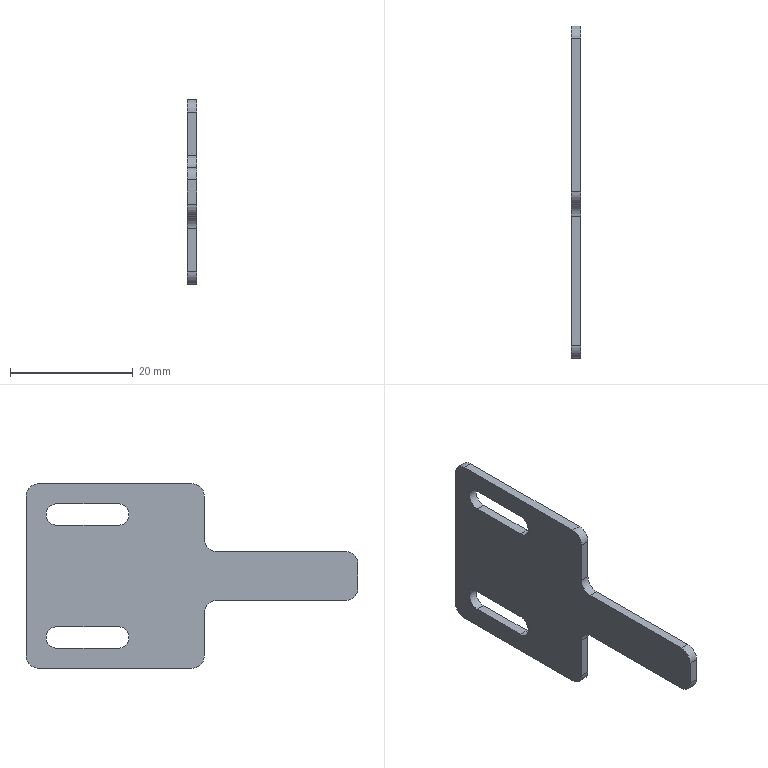Part | SolidWorks | features BaseBody 1 | 1 solid | 26 faces | box 1.5 x 54 x 30 mm | volume 1466 mm3 | plane 14 | cylinder 12 | commonest cylinder face diameters 4 x8 3.5 x4
STEP:
#1=CARTESIAN_POINT('',(-15.435,38.729,3.25));
#2=VERTEX_POINT('',#1);
#3=CARTESIAN_POINT('',(-15.435,28.729,3.25));
#4=VERTEX_POINT('',#3);
#5=CARTESIAN_POINT('',(-15.435,43.729,3.25));
#6=DIRECTION('',(0.,-1.,0.));
#7=VECTOR('',#6,1000.);
#8=LINE('',#5,#7);
#9=EDGE_CURVE('',#2,#4,#8,.T.);
#10=ORIENTED_EDGE('',*,*,#9,.F.);
#11=CARTESIAN_POINT('',(-15.435,38.729,6.75));
#12=VERTEX_POINT('',#11);
#13=CARTESIAN_POINT('',(-15.435,38.729,5.));
#14=DIRECTION('',(-1.,0.,0.));
#15=DIRECTION('',(0.,0.,-1.));
#16=AXIS2_PLACEMENT_3D('',#13,#14,#15);
#17=CIRCLE('',#16,1.75);
#18=EDGE_CURVE('',#12,#2,#17,.T.);
#19=ORIENTED_EDGE('',*,*,#18,.F.);
#20=CARTESIAN_POINT('',(-15.435,28.729,6.75));
#21=VERTEX_POINT('',#20);
#22=CARTESIAN_POINT('',(-15.435,43.729,6.75));
#23=DIRECTION('',(0.,1.,0.));
#24=VECTOR('',#23,1000.);
#25=LINE('',#22,#24);
#26=EDGE_CURVE('',#21,#12,#25,.T.);
#27=ORIENTED_EDGE('',*,*,#26,.F.);
#28=CARTESIAN_POINT('',(-15.435,28.729,5.));
#29=DIRECTION('',(-1.,0.,0.));
#30=DIRECTION('',(0.,0.,-1.));
#31=AXIS2_PLACEMENT_3D('',#28,#29,#30);
#32=CIRCLE('',#31,1.75);
#33=EDGE_CURVE('',#4,#21,#32,.T.);
#34=ORIENTED_EDGE('',*,*,#33,.F.);
#35=EDGE_LOOP('',(#10,#19,#27,#34));
#36=FACE_BOUND('',#35,.T.);
#37=CARTESIAN_POINT('',(-15.435,38.729,23.25));
#38=VERTEX_POINT('',#37);
#39=CARTESIAN_POINT('',(-15.435,28.729,23.25));
#40=VERTEX_POINT('',#39);
#41=CARTESIAN_POINT('',(-15.435,43.729,23.25));
#42=DIRECTION('',(0.,-1.,0.));
#43=VECTOR('',#42,1000.);
#44=LINE('',#41,#43);
#45=EDGE_CURVE('',#38,#40,#44,.T.);
#46=ORIENTED_EDGE('',*,*,#45,.F.);
#47=CARTESIAN_POINT('',(-15.435,38.729,26.75));
#48=VERTEX_POINT('',#47);
#49=CARTESIAN_POINT('',(-15.435,38.729,25.));
#50=DIRECTION('',(-1.,0.,0.));
#51=DIRECTION('',(0.,0.,-1.));
#52=AXIS2_PLACEMENT_3D('',#49,#50,#51);
#53=CIRCLE('',#52,1.75);
#54=EDGE_CURVE('',#48,#38,#53,.T.);
#55=ORIENTED_EDGE('',*,*,#54,.F.);
#56=CARTESIAN_POINT('',(-15.435,28.729,26.75));
#57=VERTEX_POINT('',#56);
#58=CARTESIAN_POINT('',(-15.435,43.729,26.75));
#59=DIRECTION('',(0.,1.,0.));
#60=VECTOR('',#59,1000.);
#61=LINE('',#58,#60);
#62=EDGE_CURVE('',#57,#48,#61,.T.);
#63=ORIENTED_EDGE('',*,*,#62,.F.);
#64=CARTESIAN_POINT('',(-15.435,28.729,25.));
#65=DIRECTION('',(-1.,0.,0.));
#66=DIRECTION('',(0.,0.,-1.));
#67=AXIS2_PLACEMENT_3D('',#64,#65,#66);
#68=CIRCLE('',#67,1.75);
#69=EDGE_CURVE('',#40,#57,#68,.T.);
#70=ORIENTED_EDGE('',*,*,#69,.F.);
#71=EDGE_LOOP('',(#46,#55,#63,#70));
#72=FACE_BOUND('',#71,.T.);
#73=CARTESIAN_POINT('',(-15.435,14.729,9.));
#74=VERTEX_POINT('',#73);
#75=CARTESIAN_POINT('',(-15.435,14.729,2.));
#76=VERTEX_POINT('',#75);
#77=CARTESIAN_POINT('',(-15.435,14.729,30.));
#78=DIRECTION('',(0.,0.,-1.));
#79=VECTOR('',#78,1000.);
#80=LINE('',#77,#79);
#81=EDGE_CURVE('',#74,#76,#80,.T.);
#82=ORIENTED_EDGE('',*,*,#81,.F.);
#83=CARTESIAN_POINT('',(-15.435,12.729,11.));
#84=VERTEX_POINT('',#83);
#85=CARTESIAN_POINT('',(-15.435,12.729,9.));
#86=DIRECTION('',(-1.,0.,0.));
#87=DIRECTION('',(0.,-1.,0.));
#88=AXIS2_PLACEMENT_3D('',#85,#86,#87);
#89=CIRCLE('',#88,2.);
#90=EDGE_CURVE('',#84,#74,#89,.T.);
#91=ORIENTED_EDGE('',*,*,#90,.F.);
#92=CARTESIAN_POINT('',(-15.435,-8.271,11.));
#93=VERTEX_POINT('',#92);
#94=CARTESIAN_POINT('',(-15.435,43.729,11.));
#95=DIRECTION('',(0.,1.,0.));
#96=VECTOR('',#95,1000.);
#97=LINE('',#94,#96);
#98=EDGE_CURVE('',#93,#84,#97,.T.);
#99=ORIENTED_EDGE('',*,*,#98,.F.);
#100=CARTESIAN_POINT('',(-15.435,-10.271,13.));
#101=VERTEX_POINT('',#100);
#102=CARTESIAN_POINT('',(-15.435,-8.271,13.));
#103=DIRECTION('',(1.,0.,0.));
#104=DIRECTION('',(0.,0.,-1.));
#105=AXIS2_PLACEMENT_3D('',#102,#103,#104);
#106=CIRCLE('',#105,2.);
#107=EDGE_CURVE('',#101,#93,#106,.T.);
#108=ORIENTED_EDGE('',*,*,#107,.F.);
#109=CARTESIAN_POINT('',(-15.435,-10.271,17.));
#110=VERTEX_POINT('',#109);
#111=CARTESIAN_POINT('',(-15.435,-10.271,30.));
#112=DIRECTION('',(0.,0.,-1.));
#113=VECTOR('',#112,1000.);
#114=LINE('',#111,#113);
#115=EDGE_CURVE('',#110,#101,#114,.T.);
#116=ORIENTED_EDGE('',*,*,#115,.F.);
#117=CARTESIAN_POINT('',(-15.435,-8.271,19.));
#118=VERTEX_POINT('',#117);
#119=CARTESIAN_POINT('',(-15.435,-8.271,17.));
#120=DIRECTION('',(1.,0.,0.));
#121=DIRECTION('',(0.,0.,-1.));
#122=AXIS2_PLACEMENT_3D('',#119,#120,#121);
#123=CIRCLE('',#122,2.);
#124=EDGE_CURVE('',#118,#110,#123,.T.);
#125=ORIENTED_EDGE('',*,*,#124,.F.);
#126=CARTESIAN_POINT('',(-15.435,12.729,19.));
#127=VERTEX_POINT('',#126);
#128=CARTESIAN_POINT('',(-15.435,43.729,19.));
#129=DIRECTION('',(0.,-1.,0.));
#130=VECTOR('',#129,1000.);
#131=LINE('',#128,#130);
#132=EDGE_CURVE('',#127,#118,#131,.T.);
#133=ORIENTED_EDGE('',*,*,#132,.F.);
#134=CARTESIAN_POINT('',(-15.435,14.729,21.));
#135=VERTEX_POINT('',#134);
#136=CARTESIAN_POINT('',(-15.435,12.729,21.));
#137=DIRECTION('',(-1.,0.,0.));
#138=DIRECTION('',(0.,-1.,0.));
#139=AXIS2_PLACEMENT_3D('',#136,#137,#138);
#140=CIRCLE('',#139,2.);
#141=EDGE_CURVE('',#135,#127,#140,.T.);
#142=ORIENTED_EDGE('',*,*,#141,.F.);
#143=CARTESIAN_POINT('',(-15.435,14.729,28.));
#144=VERTEX_POINT('',#143);
#145=CARTESIAN_POINT('',(-15.435,14.729,30.));
#146=DIRECTION('',(0.,0.,-1.));
#147=VECTOR('',#146,1000.);
#148=LINE('',#145,#147);
#149=EDGE_CURVE('',#144,#135,#148,.T.);
#150=ORIENTED_EDGE('',*,*,#149,.F.);
#151=CARTESIAN_POINT('',(-15.435,16.729,30.));
#152=VERTEX_POINT('',#151);
#153=CARTESIAN_POINT('',(-15.435,16.729,28.));
#154=DIRECTION('',(1.,0.,0.));
#155=DIRECTION('',(0.,1.,0.));
#156=AXIS2_PLACEMENT_3D('',#153,#154,#155);
#157=CIRCLE('',#156,2.);
#158=EDGE_CURVE('',#152,#144,#157,.T.);
#159=ORIENTED_EDGE('',*,*,#158,.F.);
#160=CARTESIAN_POINT('',(-15.435,41.729,30.));
#161=VERTEX_POINT('',#160);
#162=CARTESIAN_POINT('',(-15.435,43.729,30.));
#163=DIRECTION('',(0.,-1.,0.));
#164=VECTOR('',#163,1000.);
#165=LINE('',#162,#164);
#166=EDGE_CURVE('',#161,#152,#165,.T.);
#167=ORIENTED_EDGE('',*,*,#166,.F.);
#168=CARTESIAN_POINT('',(-15.435,43.729,28.));
#169=VERTEX_POINT('',#168);
#170=CARTESIAN_POINT('',(-15.435,41.729,28.));
#171=DIRECTION('',(1.,0.,0.));
#172=DIRECTION('',(0.,0.,1.));
#173=AXIS2_PLACEMENT_3D('',#170,#171,#172);
#174=CIRCLE('',#173,2.);
#175=EDGE_CURVE('',#169,#161,#174,.T.);
#176=ORIENTED_EDGE('',*,*,#175,.F.);
#177=CARTESIAN_POINT('',(-15.435,43.729,2.));
#178=VERTEX_POINT('',#177);
#179=CARTESIAN_POINT('',(-15.435,43.729,30.));
#180=DIRECTION('',(0.,0.,1.));
#181=VECTOR('',#180,1000.);
#182=LINE('',#179,#181);
#183=EDGE_CURVE('',#178,#169,#182,.T.);
#184=ORIENTED_EDGE('',*,*,#183,.F.);
#185=CARTESIAN_POINT('',(-15.435,41.729,0.));
#186=VERTEX_POINT('',#185);
#187=CARTESIAN_POINT('',(-15.435,41.729,2.));
#188=DIRECTION('',(1.,0.,0.));
#189=DIRECTION('',(0.,0.,-1.));
#190=AXIS2_PLACEMENT_3D('',#187,#188,#189);
#191=CIRCLE('',#190,2.);
#192=EDGE_CURVE('',#186,#178,#191,.T.);
#193=ORIENTED_EDGE('',*,*,#192,.F.);
#194=CARTESIAN_POINT('',(-15.435,16.729,0.));
#195=VERTEX_POINT('',#194);
#196=CARTESIAN_POINT('',(-15.435,43.729,0.));
#197=DIRECTION('',(0.,1.,0.));
#198=VECTOR('',#197,1000.);
#199=LINE('',#196,#198);
#200=EDGE_CURVE('',#195,#186,#199,.T.);
#201=ORIENTED_EDGE('',*,*,#200,.F.);
#202=CARTESIAN_POINT('',(-15.435,16.729,2.));
#203=DIRECTION('',(1.,0.,0.));
#204=DIRECTION('',(0.,-1.,0.));
#205=AXIS2_PLACEMENT_3D('',#202,#203,#204);
#206=CIRCLE('',#205,2.);
#207=EDGE_CURVE('',#76,#195,#206,.T.);
#208=ORIENTED_EDGE('',*,*,#207,.F.);
#209=EDGE_LOOP('',(#82,#91,#99,#108,#116,#125,#133,#142,#150,#159,#167,#176,#184,#193,#201,#208));
#210=FACE_OUTER_BOUND('',#209,.T.);
#211=CARTESIAN_POINT('',(-15.435,43.729,30.));
#212=DIRECTION('',(1.,0.,0.));
#213=DIRECTION('',(0.,1.,0.));
#214=AXIS2_PLACEMENT_3D('',#211,#212,#213);
#215=PLANE('',#214);
#216=ADVANCED_FACE('',(#36,#72,#210),#215,.F.);
#217=CARTESIAN_POINT('',(-13.935,28.729,6.75));
#218=VERTEX_POINT('',#217);
#219=CARTESIAN_POINT('',(-43.935,28.729,6.75));
#220=DIRECTION('',(-1.,0.,0.));
#221=VECTOR('',#220,1000.);
#222=LINE('',#219,#221);
#223=EDGE_CURVE('',#218,#21,#222,.T.);
#224=ORIENTED_EDGE('',*,*,#223,.F.);
#225=CARTESIAN_POINT('',(-13.935,28.729,3.25));
#226=VERTEX_POINT('',#225);
#227=CARTESIAN_POINT('',(-13.935,28.729,5.));
#228=DIRECTION('',(-1.,0.,0.));
#229=DIRECTION('',(0.,0.,-1.));
#230=AXIS2_PLACEMENT_3D('',#227,#228,#229);
#231=CIRCLE('',#230,1.75);
#232=EDGE_CURVE('',#226,#218,#231,.T.);
#233=ORIENTED_EDGE('',*,*,#232,.F.);
#234=CARTESIAN_POINT('',(-43.935,28.729,3.25));
#235=DIRECTION('',(1.,0.,0.));
#236=VECTOR('',#235,1000.);
#237=LINE('',#234,#236);
#238=EDGE_CURVE('',#4,#226,#237,.T.);
#239=ORIENTED_EDGE('',*,*,#238,.F.);
#240=ORIENTED_EDGE('',*,*,#33,.T.);
#241=EDGE_LOOP('',(#224,#233,#239,#240));
#242=FACE_OUTER_BOUND('',#241,.T.);
#243=CARTESIAN_POINT('',(-43.935,28.729,5.));
#244=DIRECTION('',(1.,0.,0.));
#245=DIRECTION('',(0.,0.,-1.));
#246=AXIS2_PLACEMENT_3D('',#243,#244,#245);
#247=CYLINDRICAL_SURFACE('',#246,1.75);
#248=ADVANCED_FACE('',(#242),#247,.F.);
#249=ORIENTED_EDGE('',*,*,#238,.T.);
#250=CARTESIAN_POINT('',(-13.935,38.729,3.25));
#251=VERTEX_POINT('',#250);
#252=CARTESIAN_POINT('',(-13.935,38.729,3.25));
#253=DIRECTION('',(0.,-1.,0.));
#254=VECTOR('',#253,1000.);
#255=LINE('',#252,#254);
#256=EDGE_CURVE('',#251,#226,#255,.T.);
#257=ORIENTED_EDGE('',*,*,#256,.F.);
#258=CARTESIAN_POINT('',(-43.935,38.729,3.25));
#259=DIRECTION('',(1.,0.,0.));
#260=VECTOR('',#259,1000.);
#261=LINE('',#258,#260);
#262=EDGE_CURVE('',#2,#251,#261,.T.);
#263=ORIENTED_EDGE('',*,*,#262,.F.);
#264=ORIENTED_EDGE('',*,*,#9,.T.);
#265=EDGE_LOOP('',(#249,#257,#263,#264));
#266=FACE_OUTER_BOUND('',#265,.T.);
#267=CARTESIAN_POINT('',(-43.935,38.729,3.25));
#268=DIRECTION('',(0.,0.,-1.));
#269=DIRECTION('',(0.,1.,0.));
#270=AXIS2_PLACEMENT_3D('',#267,#268,#269);
#271=PLANE('',#270);
#272=ADVANCED_FACE('',(#266),#271,.F.);
#273=ORIENTED_EDGE('',*,*,#262,.T.);
#274=CARTESIAN_POINT('',(-13.935,38.729,6.75));
#275=VERTEX_POINT('',#274);
#276=CARTESIAN_POINT('',(-13.935,38.729,5.));
#277=DIRECTION('',(-1.,0.,0.));
#278=DIRECTION('',(0.,0.,-1.));
#279=AXIS2_PLACEMENT_3D('',#276,#277,#278);
#280=CIRCLE('',#279,1.75);
#281=EDGE_CURVE('',#275,#251,#280,.T.);
#282=ORIENTED_EDGE('',*,*,#281,.F.);
#283=CARTESIAN_POINT('',(-43.935,38.729,6.75));
#284=DIRECTION('',(1.,0.,0.));
#285=VECTOR('',#284,1000.);
#286=LINE('',#283,#285);
#287=EDGE_CURVE('',#12,#275,#286,.T.);
#288=ORIENTED_EDGE('',*,*,#287,.F.);
#289=ORIENTED_EDGE('',*,*,#18,.T.);
#290=EDGE_LOOP('',(#273,#282,#288,#289));
#291=FACE_OUTER_BOUND('',#290,.T.);
#292=CARTESIAN_POINT('',(-43.935,38.729,5.));
#293=DIRECTION('',(1.,0.,0.));
#294=DIRECTION('',(0.,0.,-1.));
#295=AXIS2_PLACEMENT_3D('',#292,#293,#294);
#296=CYLINDRICAL_SURFACE('',#295,1.75);
#297=ADVANCED_FACE('',(#291),#296,.F.);
#298=ORIENTED_EDGE('',*,*,#287,.T.);
#299=CARTESIAN_POINT('',(-13.935,38.729,6.75));
#300=DIRECTION('',(0.,1.,0.));
#301=VECTOR('',#300,1000.);
#302=LINE('',#299,#301);
#303=EDGE_CURVE('',#218,#275,#302,.T.);
#304=ORIENTED_EDGE('',*,*,#303,.F.);
#305=ORIENTED_EDGE('',*,*,#223,.T.);
#306=ORIENTED_EDGE('',*,*,#26,.T.);
#307=EDGE_LOOP('',(#298,#304,#305,#306));
#308=FACE_OUTER_BOUND('',#307,.T.);
#309=CARTESIAN_POINT('',(-43.935,38.729,6.75));
#310=DIRECTION('',(0.,0.,1.));
#311=DIRECTION('',(0.,-1.,0.));
#312=AXIS2_PLACEMENT_3D('',#309,#310,#311);
#313=PLANE('',#312);
#314=ADVANCED_FACE('',(#308),#313,.F.);
#315=CARTESIAN_POINT('',(-13.935,28.729,26.75));
#316=VERTEX_POINT('',#315);
#317=CARTESIAN_POINT('',(-43.935,28.729,26.75));
#318=DIRECTION('',(-1.,0.,0.));
#319=VECTOR('',#318,1000.);
#320=LINE('',#317,#319);
#321=EDGE_CURVE('',#316,#57,#320,.T.);
#322=ORIENTED_EDGE('',*,*,#321,.F.);
#323=CARTESIAN_POINT('',(-13.935,28.729,23.25));
#324=VERTEX_POINT('',#323);
#325=CARTESIAN_POINT('',(-13.935,28.729,25.));
#326=DIRECTION('',(-1.,0.,0.));
#327=DIRECTION('',(0.,0.,-1.));
#328=AXIS2_PLACEMENT_3D('',#325,#326,#327);
#329=CIRCLE('',#328,1.75);
#330=EDGE_CURVE('',#324,#316,#329,.T.);
#331=ORIENTED_EDGE('',*,*,#330,.F.);
#332=CARTESIAN_POINT('',(-43.935,28.729,23.25));
#333=DIRECTION('',(1.,0.,0.));
#334=VECTOR('',#333,1000.);
#335=LINE('',#332,#334);
#336=EDGE_CURVE('',#40,#324,#335,.T.);
#337=ORIENTED_EDGE('',*,*,#336,.F.);
#338=ORIENTED_EDGE('',*,*,#69,.T.);
#339=EDGE_LOOP('',(#322,#331,#337,#338));
#340=FACE_OUTER_BOUND('',#339,.T.);
#341=CARTESIAN_POINT('',(-43.935,28.729,25.));
#342=DIRECTION('',(1.,0.,0.));
#343=DIRECTION('',(0.,0.,-1.));
#344=AXIS2_PLACEMENT_3D('',#341,#342,#343);
#345=CYLINDRICAL_SURFACE('',#344,1.75);
#346=ADVANCED_FACE('',(#340),#345,.F.);
#347=ORIENTED_EDGE('',*,*,#336,.T.);
#348=CARTESIAN_POINT('',(-13.935,38.729,23.25));
#349=VERTEX_POINT('',#348);
#350=CARTESIAN_POINT('',(-13.935,38.729,23.25));
#351=DIRECTION('',(0.,-1.,0.));
#352=VECTOR('',#351,1000.);
#353=LINE('',#350,#352);
#354=EDGE_CURVE('',#349,#324,#353,.T.);
#355=ORIENTED_EDGE('',*,*,#354,.F.);
#356=CARTESIAN_POINT('',(-43.935,38.729,23.25));
#357=DIRECTION('',(1.,0.,0.));
#358=VECTOR('',#357,1000.);
#359=LINE('',#356,#358);
#360=EDGE_CURVE('',#38,#349,#359,.T.);
#361=ORIENTED_EDGE('',*,*,#360,.F.);
#362=ORIENTED_EDGE('',*,*,#45,.T.);
#363=EDGE_LOOP('',(#347,#355,#361,#362));
#364=FACE_OUTER_BOUND('',#363,.T.);
#365=CARTESIAN_POINT('',(-43.935,38.729,23.25));
#366=DIRECTION('',(0.,0.,-1.));
#367=DIRECTION('',(0.,1.,0.));
#368=AXIS2_PLACEMENT_3D('',#365,#366,#367);
#369=PLANE('',#368);
#370=ADVANCED_FACE('',(#364),#369,.F.);
#371=ORIENTED_EDGE('',*,*,#360,.T.);
#372=CARTESIAN_POINT('',(-13.935,38.729,26.75));
#373=VERTEX_POINT('',#372);
#374=CARTESIAN_POINT('',(-13.935,38.729,25.));
#375=DIRECTION('',(-1.,0.,0.));
#376=DIRECTION('',(0.,0.,-1.));
#377=AXIS2_PLACEMENT_3D('',#374,#375,#376);
#378=CIRCLE('',#377,1.75);
#379=EDGE_CURVE('',#373,#349,#378,.T.);
#380=ORIENTED_EDGE('',*,*,#379,.F.);
#381=CARTESIAN_POINT('',(-43.935,38.729,26.75));
#382=DIRECTION('',(1.,0.,0.));
#383=VECTOR('',#382,1000.);
#384=LINE('',#381,#383);
#385=EDGE_CURVE('',#48,#373,#384,.T.);
#386=ORIENTED_EDGE('',*,*,#385,.F.);
#387=ORIENTED_EDGE('',*,*,#54,.T.);
#388=EDGE_LOOP('',(#371,#380,#386,#387));
#389=FACE_OUTER_BOUND('',#388,.T.);
#390=CARTESIAN_POINT('',(-43.935,38.729,25.));
#391=DIRECTION('',(1.,0.,0.));
#392=DIRECTION('',(0.,0.,-1.));
#393=AXIS2_PLACEMENT_3D('',#390,#391,#392);
#394=CYLINDRICAL_SURFACE('',#393,1.75);
#395=ADVANCED_FACE('',(#389),#394,.F.);
#396=ORIENTED_EDGE('',*,*,#385,.T.);
#397=CARTESIAN_POINT('',(-13.935,38.729,26.75));
#398=DIRECTION('',(0.,1.,0.));
#399=VECTOR('',#398,1000.);
#400=LINE('',#397,#399);
#401=EDGE_CURVE('',#316,#373,#400,.T.);
#402=ORIENTED_EDGE('',*,*,#401,.F.);
#403=ORIENTED_EDGE('',*,*,#321,.T.);
#404=ORIENTED_EDGE('',*,*,#62,.T.);
#405=EDGE_LOOP('',(#396,#402,#403,#404));
#406=FACE_OUTER_BOUND('',#405,.T.);
#407=CARTESIAN_POINT('',(-43.935,38.729,26.75));
#408=DIRECTION('',(0.,0.,1.));
#409=DIRECTION('',(0.,-1.,0.));
#410=AXIS2_PLACEMENT_3D('',#407,#408,#409);
#411=PLANE('',#410);
#412=ADVANCED_FACE('',(#406),#411,.F.);
#413=ORIENTED_EDGE('',*,*,#207,.T.);
#414=CARTESIAN_POINT('',(-13.935,16.729,0.));
#415=VERTEX_POINT('',#414);
#416=CARTESIAN_POINT('',(-23.935,16.729,0.));
#417=DIRECTION('',(1.,0.,0.));
#418=VECTOR('',#417,1000.);
#419=LINE('',#416,#418);
#420=EDGE_CURVE('',#195,#415,#419,.T.);
#421=ORIENTED_EDGE('',*,*,#420,.T.);
#422=CARTESIAN_POINT('',(-13.935,14.729,2.));
#423=VERTEX_POINT('',#422);
#424=CARTESIAN_POINT('',(-13.935,16.729,2.));
#425=DIRECTION('',(-1.,0.,0.));
#426=DIRECTION('',(0.,-1.,0.));
#427=AXIS2_PLACEMENT_3D('',#424,#425,#426);
#428=CIRCLE('',#427,2.);
#429=EDGE_CURVE('',#415,#423,#428,.T.);
#430=ORIENTED_EDGE('',*,*,#429,.T.);
#431=CARTESIAN_POINT('',(-23.935,14.729,2.));
#432=DIRECTION('',(-1.,0.,0.));
#433=VECTOR('',#432,1000.);
#434=LINE('',#431,#433);
#435=EDGE_CURVE('',#423,#76,#434,.T.);
#436=ORIENTED_EDGE('',*,*,#435,.T.);
#437=EDGE_LOOP('',(#413,#421,#430,#436));
#438=FACE_OUTER_BOUND('',#437,.T.);
#439=CARTESIAN_POINT('',(-23.935,16.729,2.));
#440=DIRECTION('',(-1.,0.,0.));
#441=DIRECTION('',(0.,-1.,0.));
#442=AXIS2_PLACEMENT_3D('',#439,#440,#441);
#443=CYLINDRICAL_SURFACE('',#442,2.);
#444=ADVANCED_FACE('',(#438),#443,.T.);
#445=ORIENTED_EDGE('',*,*,#81,.T.);
#446=ORIENTED_EDGE('',*,*,#435,.F.);
#447=CARTESIAN_POINT('',(-13.935,14.729,9.));
#448=VERTEX_POINT('',#447);
#449=CARTESIAN_POINT('',(-13.935,14.729,0.));
#450=DIRECTION('',(0.,0.,-1.));
#451=VECTOR('',#450,1000.);
#452=LINE('',#449,#451);
#453=EDGE_CURVE('',#448,#423,#452,.T.);
#454=ORIENTED_EDGE('',*,*,#453,.F.);
#455=CARTESIAN_POINT('',(-23.935,14.729,9.));
#456=DIRECTION('',(1.,0.,0.));
#457=VECTOR('',#456,1000.);
#458=LINE('',#455,#457);
#459=EDGE_CURVE('',#74,#448,#458,.T.);
#460=ORIENTED_EDGE('',*,*,#459,.F.);
#461=EDGE_LOOP('',(#445,#446,#454,#460));
#462=FACE_OUTER_BOUND('',#461,.T.);
#463=CARTESIAN_POINT('',(-23.935,14.729,0.));
#464=DIRECTION('',(0.,1.,0.));
#465=DIRECTION('',(0.,0.,1.));
#466=AXIS2_PLACEMENT_3D('',#463,#464,#465);
#467=PLANE('',#466);
#468=ADVANCED_FACE('',(#462),#467,.F.);
#469=ORIENTED_EDGE('',*,*,#90,.T.);
#470=ORIENTED_EDGE('',*,*,#459,.T.);
#471=CARTESIAN_POINT('',(-13.935,12.729,11.));
#472=VERTEX_POINT('',#471);
#473=CARTESIAN_POINT('',(-13.935,12.729,9.));
#474=DIRECTION('',(-1.,0.,0.));
#475=DIRECTION('',(0.,-1.,0.));
#476=AXIS2_PLACEMENT_3D('',#473,#474,#475);
#477=CIRCLE('',#476,2.);
#478=EDGE_CURVE('',#472,#448,#477,.T.);
#479=ORIENTED_EDGE('',*,*,#478,.F.);
#480=CARTESIAN_POINT('',(-23.935,12.729,11.));
#481=DIRECTION('',(1.,0.,0.));
#482=VECTOR('',#481,1000.);
#483=LINE('',#480,#482);
#484=EDGE_CURVE('',#84,#472,#483,.T.);
#485=ORIENTED_EDGE('',*,*,#484,.F.);
#486=EDGE_LOOP('',(#469,#470,#479,#485));
#487=FACE_OUTER_BOUND('',#486,.T.);
#488=CARTESIAN_POINT('',(-23.935,12.729,9.));
#489=DIRECTION('',(-1.,0.,0.));
#490=DIRECTION('',(0.,-1.,0.));
#491=AXIS2_PLACEMENT_3D('',#488,#489,#490);
#492=CYLINDRICAL_SURFACE('',#491,2.);
#493=ADVANCED_FACE('',(#487),#492,.F.);
#494=ORIENTED_EDGE('',*,*,#98,.T.);
#495=ORIENTED_EDGE('',*,*,#484,.T.);
#496=CARTESIAN_POINT('',(-13.935,-8.271,11.));
#497=VERTEX_POINT('',#496);
#498=CARTESIAN_POINT('',(-13.935,-10.271,11.));
#499=DIRECTION('',(0.,1.,0.));
#500=VECTOR('',#499,1000.);
#501=LINE('',#498,#500);
#502=EDGE_CURVE('',#497,#472,#501,.T.);
#503=ORIENTED_EDGE('',*,*,#502,.F.);
#504=CARTESIAN_POINT('',(-23.935,-8.271,11.));
#505=DIRECTION('',(1.,0.,0.));
#506=VECTOR('',#505,1000.);
#507=LINE('',#504,#506);
#508=EDGE_CURVE('',#93,#497,#507,.T.);
#509=ORIENTED_EDGE('',*,*,#508,.F.);
#510=EDGE_LOOP('',(#494,#495,#503,#509));
#511=FACE_OUTER_BOUND('',#510,.T.);
#512=CARTESIAN_POINT('',(-23.935,-10.271,11.));
#513=DIRECTION('',(0.,0.,1.));
#514=DIRECTION('',(1.,0.,0.));
#515=AXIS2_PLACEMENT_3D('',#512,#513,#514);
#516=PLANE('',#515);
#517=ADVANCED_FACE('',(#511),#516,.F.);
#518=ORIENTED_EDGE('',*,*,#107,.T.);
#519=ORIENTED_EDGE('',*,*,#508,.T.);
#520=CARTESIAN_POINT('',(-13.935,-10.271,13.));
#521=VERTEX_POINT('',#520);
#522=CARTESIAN_POINT('',(-13.935,-8.271,13.));
#523=DIRECTION('',(-1.,0.,0.));
#524=DIRECTION('',(0.,0.,-1.));
#525=AXIS2_PLACEMENT_3D('',#522,#523,#524);
#526=CIRCLE('',#525,2.);
#527=EDGE_CURVE('',#497,#521,#526,.T.);
#528=ORIENTED_EDGE('',*,*,#527,.T.);
#529=CARTESIAN_POINT('',(-13.935,-10.271,13.));
#530=DIRECTION('',(-1.,0.,0.));
#531=VECTOR('',#530,1000.);
#532=LINE('',#529,#531);
#533=EDGE_CURVE('',#521,#101,#532,.T.);
#534=ORIENTED_EDGE('',*,*,#533,.T.);
#535=EDGE_LOOP('',(#518,#519,#528,#534));
#536=FACE_OUTER_BOUND('',#535,.T.);
#537=CARTESIAN_POINT('',(-13.935,-8.271,13.));
#538=DIRECTION('',(1.,0.,0.));
#539=DIRECTION('',(0.,0.,-1.));
#540=AXIS2_PLACEMENT_3D('',#537,#538,#539);
#541=CYLINDRICAL_SURFACE('',#540,2.);
#542=ADVANCED_FACE('',(#536),#541,.T.);
#543=ORIENTED_EDGE('',*,*,#115,.T.);
#544=ORIENTED_EDGE('',*,*,#533,.F.);
#545=CARTESIAN_POINT('',(-13.935,-10.271,17.));
#546=VERTEX_POINT('',#545);
#547=CARTESIAN_POINT('',(-13.935,-10.271,30.));
#548=DIRECTION('',(0.,0.,-1.));
#549=VECTOR('',#548,1000.);
#550=LINE('',#547,#549);
#551=EDGE_CURVE('',#546,#521,#550,.T.);
#552=ORIENTED_EDGE('',*,*,#551,.F.);
#553=CARTESIAN_POINT('',(-13.935,-10.271,17.));
#554=DIRECTION('',(1.,0.,0.));
#555=VECTOR('',#554,1000.);
#556=LINE('',#553,#555);
#557=EDGE_CURVE('',#110,#546,#556,.T.);
#558=ORIENTED_EDGE('',*,*,#557,.F.);
#559=EDGE_LOOP('',(#543,#544,#552,#558));
#560=FACE_OUTER_BOUND('',#559,.T.);
#561=CARTESIAN_POINT('',(-13.935,-10.271,30.));
#562=DIRECTION('',(0.,1.,0.));
#563=DIRECTION('',(0.,0.,1.));
#564=AXIS2_PLACEMENT_3D('',#561,#562,#563);
#565=PLANE('',#564);
#566=ADVANCED_FACE('',(#560),#565,.F.);
#567=ORIENTED_EDGE('',*,*,#124,.T.);
#568=ORIENTED_EDGE('',*,*,#557,.T.);
#569=CARTESIAN_POINT('',(-13.935,-8.271,19.));
#570=VERTEX_POINT('',#569);
#571=CARTESIAN_POINT('',(-13.935,-8.271,17.));
#572=DIRECTION('',(-1.,0.,0.));
#573=DIRECTION('',(0.,0.,-1.));
#574=AXIS2_PLACEMENT_3D('',#571,#572,#573);
#575=CIRCLE('',#574,2.);
#576=EDGE_CURVE('',#546,#570,#575,.T.);
#577=ORIENTED_EDGE('',*,*,#576,.T.);
#578=CARTESIAN_POINT('',(-23.935,-8.271,19.));
#579=DIRECTION('',(-1.,0.,0.));
#580=VECTOR('',#579,1000.);
#581=LINE('',#578,#580);
#582=EDGE_CURVE('',#570,#118,#581,.T.);
#583=ORIENTED_EDGE('',*,*,#582,.T.);
#584=EDGE_LOOP('',(#567,#568,#577,#583));
#585=FACE_OUTER_BOUND('',#584,.T.);
#586=CARTESIAN_POINT('',(-23.935,-8.271,17.));
#587=DIRECTION('',(1.,0.,0.));
#588=DIRECTION('',(0.,0.,-1.));
#589=AXIS2_PLACEMENT_3D('',#586,#587,#588);
#590=CYLINDRICAL_SURFACE('',#589,2.);
#591=ADVANCED_FACE('',(#585),#590,.T.);
#592=CARTESIAN_POINT('',(-13.935,12.729,19.));
#593=VERTEX_POINT('',#592);
#594=CARTESIAN_POINT('',(-13.935,-10.271,19.));
#595=DIRECTION('',(0.,-1.,0.));
#596=VECTOR('',#595,1000.);
#597=LINE('',#594,#596);
#598=EDGE_CURVE('',#593,#570,#597,.T.);
#599=ORIENTED_EDGE('',*,*,#598,.F.);
#600=CARTESIAN_POINT('',(-23.935,12.729,19.));
#601=DIRECTION('',(1.,0.,0.));
#602=VECTOR('',#601,1000.);
#603=LINE('',#600,#602);
#604=EDGE_CURVE('',#127,#593,#603,.T.);
#605=ORIENTED_EDGE('',*,*,#604,.F.);
#606=ORIENTED_EDGE('',*,*,#132,.T.);
#607=ORIENTED_EDGE('',*,*,#582,.F.);
#608=EDGE_LOOP('',(#599,#605,#606,#607));
#609=FACE_OUTER_BOUND('',#608,.T.);
#610=CARTESIAN_POINT('',(-23.935,-10.271,19.));
#611=DIRECTION('',(0.,0.,-1.));
#612=DIRECTION('',(-1.,0.,0.));
#613=AXIS2_PLACEMENT_3D('',#610,#611,#612);
#614=PLANE('',#613);
#615=ADVANCED_FACE('',(#609),#614,.F.);
#616=ORIENTED_EDGE('',*,*,#141,.T.);
#617=ORIENTED_EDGE('',*,*,#604,.T.);
#618=CARTESIAN_POINT('',(-13.935,14.729,21.));
#619=VERTEX_POINT('',#618);
#620=CARTESIAN_POINT('',(-13.935,12.729,21.));
#621=DIRECTION('',(-1.,0.,0.));
#622=DIRECTION('',(0.,-1.,0.));
#623=AXIS2_PLACEMENT_3D('',#620,#621,#622);
#624=CIRCLE('',#623,2.);
#625=EDGE_CURVE('',#619,#593,#624,.T.);
#626=ORIENTED_EDGE('',*,*,#625,.F.);
#627=CARTESIAN_POINT('',(-23.935,14.729,21.));
#628=DIRECTION('',(1.,0.,0.));
#629=VECTOR('',#628,1000.);
#630=LINE('',#627,#629);
#631=EDGE_CURVE('',#135,#619,#630,.T.);
#632=ORIENTED_EDGE('',*,*,#631,.F.);
#633=EDGE_LOOP('',(#616,#617,#626,#632));
#634=FACE_OUTER_BOUND('',#633,.T.);
#635=CARTESIAN_POINT('',(-23.935,12.729,21.));
#636=DIRECTION('',(-1.,0.,0.));
#637=DIRECTION('',(0.,-1.,0.));
#638=AXIS2_PLACEMENT_3D('',#635,#636,#637);
#639=CYLINDRICAL_SURFACE('',#638,2.);
#640=ADVANCED_FACE('',(#634),#639,.F.);
#641=CARTESIAN_POINT('',(-13.935,14.729,28.));
#642=VERTEX_POINT('',#641);
#643=CARTESIAN_POINT('',(-13.935,14.729,30.));
#644=DIRECTION('',(0.,0.,-1.));
#645=VECTOR('',#644,1000.);
#646=LINE('',#643,#645);
#647=EDGE_CURVE('',#642,#619,#646,.T.);
#648=ORIENTED_EDGE('',*,*,#647,.F.);
#649=CARTESIAN_POINT('',(-23.935,14.729,28.));
#650=DIRECTION('',(1.,0.,0.));
#651=VECTOR('',#650,1000.);
#652=LINE('',#649,#651);
#653=EDGE_CURVE('',#144,#642,#652,.T.);
#654=ORIENTED_EDGE('',*,*,#653,.F.);
#655=ORIENTED_EDGE('',*,*,#149,.T.);
#656=ORIENTED_EDGE('',*,*,#631,.T.);
#657=EDGE_LOOP('',(#648,#654,#655,#656));
#658=FACE_OUTER_BOUND('',#657,.T.);
#659=CARTESIAN_POINT('',(-23.935,14.729,30.));
#660=DIRECTION('',(0.,1.,0.));
#661=DIRECTION('',(-1.,0.,0.));
#662=AXIS2_PLACEMENT_3D('',#659,#660,#661);
#663=PLANE('',#662);
#664=ADVANCED_FACE('',(#658),#663,.F.);
#665=ORIENTED_EDGE('',*,*,#158,.T.);
#666=ORIENTED_EDGE('',*,*,#653,.T.);
#667=CARTESIAN_POINT('',(-13.935,16.729,30.));
#668=VERTEX_POINT('',#667);
#669=CARTESIAN_POINT('',(-13.935,16.729,28.));
#670=DIRECTION('',(-1.,0.,0.));
#671=DIRECTION('',(0.,1.,0.));
#672=AXIS2_PLACEMENT_3D('',#669,#670,#671);
#673=CIRCLE('',#672,2.);
#674=EDGE_CURVE('',#642,#668,#673,.T.);
#675=ORIENTED_EDGE('',*,*,#674,.T.);
#676=CARTESIAN_POINT('',(0.,16.729,30.));
#677=DIRECTION('',(-1.,0.,0.));
#678=VECTOR('',#677,1000.);
#679=LINE('',#676,#678);
#680=EDGE_CURVE('',#668,#152,#679,.T.);
#681=ORIENTED_EDGE('',*,*,#680,.T.);
#682=EDGE_LOOP('',(#665,#666,#675,#681));
#683=FACE_OUTER_BOUND('',#682,.T.);
#684=CARTESIAN_POINT('',(0.,16.729,28.));
#685=DIRECTION('',(1.,0.,0.));
#686=DIRECTION('',(0.,1.,0.));
#687=AXIS2_PLACEMENT_3D('',#684,#685,#686);
#688=CYLINDRICAL_SURFACE('',#687,2.);
#689=ADVANCED_FACE('',(#683),#688,.T.);
#690=CARTESIAN_POINT('',(-13.935,41.729,30.));
#691=VERTEX_POINT('',#690);
#692=CARTESIAN_POINT('',(-13.935,0.,30.));
#693=DIRECTION('',(0.,-1.,0.));
#694=VECTOR('',#693,1000.);
#695=LINE('',#692,#694);
#696=EDGE_CURVE('',#691,#668,#695,.T.);
#697=ORIENTED_EDGE('',*,*,#696,.F.);
#698=CARTESIAN_POINT('',(0.,41.729,30.));
#699=DIRECTION('',(1.,0.,0.));
#700=VECTOR('',#699,1000.);
#701=LINE('',#698,#700);
#702=EDGE_CURVE('',#161,#691,#701,.T.);
#703=ORIENTED_EDGE('',*,*,#702,.F.);
#704=ORIENTED_EDGE('',*,*,#166,.T.);
#705=ORIENTED_EDGE('',*,*,#680,.F.);
#706=EDGE_LOOP('',(#697,#703,#704,#705));
#707=FACE_OUTER_BOUND('',#706,.T.);
#708=CARTESIAN_POINT('',(0.,0.,30.));
#709=DIRECTION('',(0.,0.,-1.));
#710=DIRECTION('',(-1.,0.,0.));
#711=AXIS2_PLACEMENT_3D('',#708,#709,#710);
#712=PLANE('',#711);
#713=ADVANCED_FACE('',(#707),#712,.F.);
#714=CARTESIAN_POINT('',(-13.935,43.729,28.));
#715=VERTEX_POINT('',#714);
#716=CARTESIAN_POINT('',(-13.935,41.729,28.));
#717=DIRECTION('',(-1.,0.,0.));
#718=DIRECTION('',(0.,0.,1.));
#719=AXIS2_PLACEMENT_3D('',#716,#717,#718);
#720=CIRCLE('',#719,2.);
#721=EDGE_CURVE('',#691,#715,#720,.T.);
#722=ORIENTED_EDGE('',*,*,#721,.T.);
#723=CARTESIAN_POINT('',(0.,43.729,28.));
#724=DIRECTION('',(-1.,0.,0.));
#725=VECTOR('',#724,1000.);
#726=LINE('',#723,#725);
#727=EDGE_CURVE('',#715,#169,#726,.T.);
#728=ORIENTED_EDGE('',*,*,#727,.T.);
#729=ORIENTED_EDGE('',*,*,#175,.T.);
#730=ORIENTED_EDGE('',*,*,#702,.T.);
#731=EDGE_LOOP('',(#722,#728,#729,#730));
#732=FACE_OUTER_BOUND('',#731,.T.);
#733=CARTESIAN_POINT('',(0.,41.729,28.));
#734=DIRECTION('',(-1.,0.,0.));
#735=DIRECTION('',(0.,0.,1.));
#736=AXIS2_PLACEMENT_3D('',#733,#734,#735);
#737=CYLINDRICAL_SURFACE('',#736,2.);
#738=ADVANCED_FACE('',(#732),#737,.T.);
#739=CARTESIAN_POINT('',(-13.935,43.729,2.));
#740=VERTEX_POINT('',#739);
#741=CARTESIAN_POINT('',(-13.935,43.729,30.));
#742=DIRECTION('',(0.,0.,1.));
#743=VECTOR('',#742,1000.);
#744=LINE('',#741,#743);
#745=EDGE_CURVE('',#740,#715,#744,.T.);
#746=ORIENTED_EDGE('',*,*,#745,.F.);
#747=CARTESIAN_POINT('',(-15.435,43.729,2.));
#748=DIRECTION('',(1.,0.,0.));
#749=VECTOR('',#748,1000.);
#750=LINE('',#747,#749);
#751=EDGE_CURVE('',#178,#740,#750,.T.);
#752=ORIENTED_EDGE('',*,*,#751,.F.);
#753=ORIENTED_EDGE('',*,*,#183,.T.);
#754=ORIENTED_EDGE('',*,*,#727,.F.);
#755=EDGE_LOOP('',(#746,#752,#753,#754));
#756=FACE_OUTER_BOUND('',#755,.T.);
#757=CARTESIAN_POINT('',(-15.435,43.729,30.));
#758=DIRECTION('',(0.,-1.,0.));
#759=DIRECTION('',(0.,0.,-1.));
#760=AXIS2_PLACEMENT_3D('',#757,#758,#759);
#761=PLANE('',#760);
#762=ADVANCED_FACE('',(#756),#761,.F.);
#763=CARTESIAN_POINT('',(-13.935,41.729,0.));
#764=VERTEX_POINT('',#763);
#765=CARTESIAN_POINT('',(-13.935,41.729,2.));
#766=DIRECTION('',(-1.,0.,0.));
#767=DIRECTION('',(0.,0.,-1.));
#768=AXIS2_PLACEMENT_3D('',#765,#766,#767);
#769=CIRCLE('',#768,2.);
#770=EDGE_CURVE('',#740,#764,#769,.T.);
#771=ORIENTED_EDGE('',*,*,#770,.T.);
#772=CARTESIAN_POINT('',(-15.435,41.729,0.));
#773=DIRECTION('',(-1.,0.,0.));
#774=VECTOR('',#773,1000.);
#775=LINE('',#772,#774);
#776=EDGE_CURVE('',#764,#186,#775,.T.);
#777=ORIENTED_EDGE('',*,*,#776,.T.);
#778=ORIENTED_EDGE('',*,*,#192,.T.);
#779=ORIENTED_EDGE('',*,*,#751,.T.);
#780=EDGE_LOOP('',(#771,#777,#778,#779));
#781=FACE_OUTER_BOUND('',#780,.T.);
#782=CARTESIAN_POINT('',(-15.435,41.729,2.));
#783=DIRECTION('',(1.,0.,0.));
#784=DIRECTION('',(0.,0.,-1.));
#785=AXIS2_PLACEMENT_3D('',#782,#783,#784);
#786=CYLINDRICAL_SURFACE('',#785,2.);
#787=ADVANCED_FACE('',(#781),#786,.T.);
#788=ORIENTED_EDGE('',*,*,#200,.T.);
#789=ORIENTED_EDGE('',*,*,#776,.F.);
#790=CARTESIAN_POINT('',(-13.935,0.,0.));
#791=DIRECTION('',(0.,-1.,0.));
#792=VECTOR('',#791,1000.);
#793=LINE('',#790,#792);
#794=EDGE_CURVE('',#764,#415,#793,.T.);
#795=ORIENTED_EDGE('',*,*,#794,.T.);
#796=ORIENTED_EDGE('',*,*,#420,.F.);
#797=EDGE_LOOP('',(#788,#789,#795,#796));
#798=FACE_OUTER_BOUND('',#797,.T.);
#799=CARTESIAN_POINT('',(0.,0.,0.));
#800=DIRECTION('',(0.,0.,-1.));
#801=DIRECTION('',(-1.,0.,0.));
#802=AXIS2_PLACEMENT_3D('',#799,#800,#801);
#803=PLANE('',#802);
#804=ADVANCED_FACE('',(#798),#803,.T.);
#805=ORIENTED_EDGE('',*,*,#303,.T.);
#806=ORIENTED_EDGE('',*,*,#281,.T.);
#807=ORIENTED_EDGE('',*,*,#256,.T.);
#808=ORIENTED_EDGE('',*,*,#232,.T.);
#809=EDGE_LOOP('',(#805,#806,#807,#808));
#810=FACE_BOUND('',#809,.T.);
#811=ORIENTED_EDGE('',*,*,#401,.T.);
#812=ORIENTED_EDGE('',*,*,#379,.T.);
#813=ORIENTED_EDGE('',*,*,#354,.T.);
#814=ORIENTED_EDGE('',*,*,#330,.T.);
#815=EDGE_LOOP('',(#811,#812,#813,#814));
#816=FACE_BOUND('',#815,.T.);
#817=ORIENTED_EDGE('',*,*,#696,.T.);
#818=ORIENTED_EDGE('',*,*,#674,.F.);
#819=ORIENTED_EDGE('',*,*,#647,.T.);
#820=ORIENTED_EDGE('',*,*,#625,.T.);
#821=ORIENTED_EDGE('',*,*,#598,.T.);
#822=ORIENTED_EDGE('',*,*,#576,.F.);
#823=ORIENTED_EDGE('',*,*,#551,.T.);
#824=ORIENTED_EDGE('',*,*,#527,.F.);
#825=ORIENTED_EDGE('',*,*,#502,.T.);
#826=ORIENTED_EDGE('',*,*,#478,.T.);
#827=ORIENTED_EDGE('',*,*,#453,.T.);
#828=ORIENTED_EDGE('',*,*,#429,.F.);
#829=ORIENTED_EDGE('',*,*,#794,.F.);
#830=ORIENTED_EDGE('',*,*,#770,.F.);
#831=ORIENTED_EDGE('',*,*,#745,.T.);
#832=ORIENTED_EDGE('',*,*,#721,.F.);
#833=EDGE_LOOP('',(#817,#818,#819,#820,#821,#822,#823,#824,#825,#826,#827,#828,#829,#830,#831,#832));
#834=FACE_OUTER_BOUND('',#833,.T.);
#835=CARTESIAN_POINT('',(-13.935,43.729,30.));
#836=DIRECTION('',(-1.,0.,0.));
#837=DIRECTION('',(0.,-1.,0.));
#838=AXIS2_PLACEMENT_3D('',#835,#836,#837);
#839=PLANE('',#838);
#840=ADVANCED_FACE('',(#810,#816,#834),#839,.F.);
#841=CLOSED_SHELL('',(#216,#248,#272,#297,#314,#346,#370,#395,#412,#444,#468,#493,#517,#542,#566,#591,#615,#640,#664,#689,#713,#738,#762,#787,#804,#840));
#842=MANIFOLD_SOLID_BREP('',#841);
#843=CARTESIAN_POINT('',(0.,0.,0.));
#844=DIRECTION('',(0.,0.,1.));
#845=DIRECTION('',(1.,0.,0.));
#846=AXIS2_PLACEMENT_3D('',#843,#844,#845);
#847=(LENGTH_UNIT()NAMED_UNIT(*)SI_UNIT(.MILLI.,.METRE.));
#848=UNCERTAINTY_MEASURE_WITH_UNIT(LENGTH_MEASURE(0.00001),#847,'','');
#849=(NAMED_UNIT(*)PLANE_ANGLE_UNIT()SI_UNIT($,.RADIAN.));
#850=(NAMED_UNIT(*)SI_UNIT($,.STERADIAN.)SOLID_ANGLE_UNIT());
#851=(GEOMETRIC_REPRESENTATION_CONTEXT(3)GLOBAL_UNCERTAINTY_ASSIGNED_CONTEXT((#848))GLOBAL_UNIT_ASSIGNED_CONTEXT((#847,#849,#850))REPRESENTATION_CONTEXT('',''));
#852=ADVANCED_BREP_SHAPE_REPRESENTATION('',(#842,#846),#851);